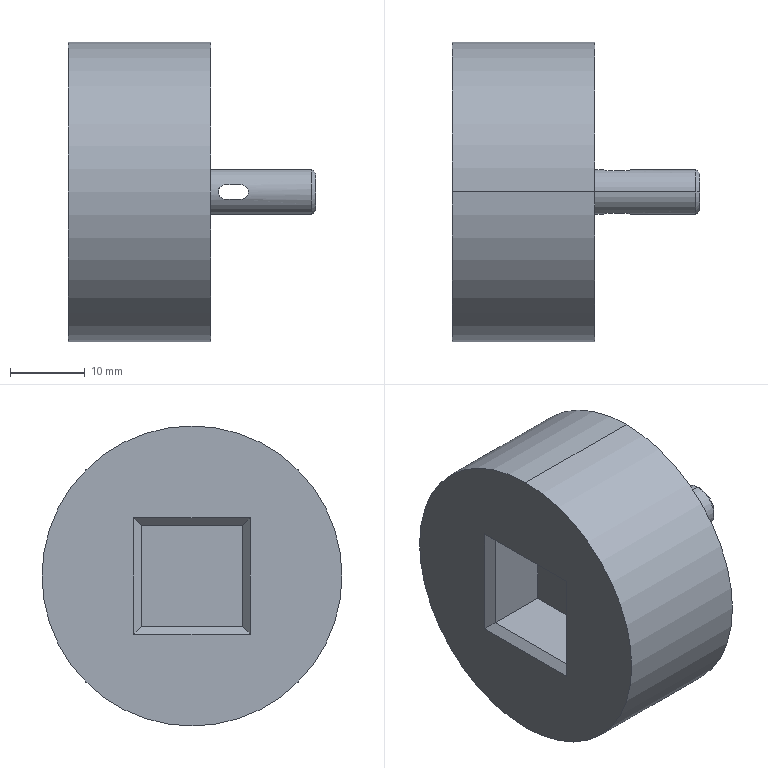Part | SolidWorks | features Chamfer 2, ICE 2, Revolution 1 | 1 solid | 22 faces | box 33 x 40 x 40 mm | volume 22559 mm3 | plane 14 | cylinder 6 | cone 2 | commonest cylinder face diameters 2 x2 6 x2 40 x2
STEP:
#1=CARTESIAN_POINT('',(14.,0.,-2.5));
#2=VERTEX_POINT('',#1);
#3=CARTESIAN_POINT('',(14.,0.,2.5));
#4=VERTEX_POINT('',#3);
#5=CARTESIAN_POINT('',(14.,0.,0.));
#6=DIRECTION('',(1.,0.,0.));
#7=DIRECTION('',(0.,0.,-1.));
#8=AXIS2_PLACEMENT_3D('',#5,#6,#7);
#9=CIRCLE('',#8,2.5);
#10=EDGE_CURVE('',#2,#4,#9,.T.);
#11=ORIENTED_EDGE('',*,*,#10,.F.);
#12=CARTESIAN_POINT('',(13.5,0.,-3.));
#13=VERTEX_POINT('',#12);
#14=CARTESIAN_POINT('',(13.5,0.,-3.));
#15=DIRECTION('',(-0.7071,0.,-0.7071));
#16=VECTOR('',#15,1000.);
#17=LINE('',#14,#16);
#18=EDGE_CURVE('',#2,#13,#17,.T.);
#19=ORIENTED_EDGE('',*,*,#18,.T.);
#20=CARTESIAN_POINT('',(13.5,0.,3.));
#21=VERTEX_POINT('',#20);
#22=CARTESIAN_POINT('',(13.5,0.,0.));
#23=DIRECTION('',(-1.,0.,0.));
#24=DIRECTION('',(0.,0.,-1.));
#25=AXIS2_PLACEMENT_3D('',#22,#23,#24);
#26=CIRCLE('',#25,3.);
#27=EDGE_CURVE('',#21,#13,#26,.T.);
#28=ORIENTED_EDGE('',*,*,#27,.F.);
#29=CARTESIAN_POINT('',(13.5,0.,3.));
#30=DIRECTION('',(-0.7071,0.,0.7071));
#31=VECTOR('',#30,1000.);
#32=LINE('',#29,#31);
#33=EDGE_CURVE('',#4,#21,#32,.T.);
#34=ORIENTED_EDGE('',*,*,#33,.F.);
#35=EDGE_LOOP('',(#11,#19,#28,#34));
#36=FACE_OUTER_BOUND('',#35,.T.);
#37=CARTESIAN_POINT('',(13.5,0.,0.));
#38=DIRECTION('',(-1.,0.,0.));
#39=DIRECTION('',(0.,0.,1.));
#40=AXIS2_PLACEMENT_3D('',#37,#38,#39);
#41=CONICAL_SURFACE('',#40,3.,0.7854);
#42=ADVANCED_FACE('',(#36),#41,.T.);
#43=CARTESIAN_POINT('',(2.,2.828,-1.));
#44=VERTEX_POINT('',#43);
#45=CARTESIAN_POINT('',(2.,2.828,1.));
#46=VERTEX_POINT('',#45);
#47=CARTESIAN_POINT('',(2.,2.828,-1.));
#48=CARTESIAN_POINT('',(1.867,2.828,-1.));
#49=CARTESIAN_POINT('',(1.736,2.838,-0.9735));
#50=CARTESIAN_POINT('',(1.495,2.871,-0.8728));
#51=CARTESIAN_POINT('',(1.384,2.893,-0.7987));
#52=CARTESIAN_POINT('',(1.201,2.938,-0.6157));
#53=CARTESIAN_POINT('',(1.127,2.96,-0.505));
#54=CARTESIAN_POINT('',(1.027,2.991,-0.2647));
#55=CARTESIAN_POINT('',(1.,3.,-0.1326));
#56=CARTESIAN_POINT('',(0.9999,3.,0.1304));
#57=CARTESIAN_POINT('',(1.026,2.991,0.2619));
#58=CARTESIAN_POINT('',(1.127,2.96,0.5053));
#59=CARTESIAN_POINT('',(1.201,2.938,0.6149));
#60=CARTESIAN_POINT('',(1.385,2.893,0.799));
#61=CARTESIAN_POINT('',(1.495,2.871,0.8728));
#62=CARTESIAN_POINT('',(1.735,2.838,0.9731));
#63=CARTESIAN_POINT('',(1.867,2.828,1.));
#64=CARTESIAN_POINT('',(2.,2.828,1.));
#65=B_SPLINE_CURVE_WITH_KNOTS('',3,(#47,#48,#49,#50,#51,#52,#53,#54,#55,#56,#57,#58,#59,#60,#61,#62,#63,#64),.UNSPECIFIED.,.F.,.F.,(4,2,2,2,2,2,2,2,4),(0.,0.0003935,0.000787,0.00118,0.001574,0.001967,0.002361,0.002754,0.003148),.UNSPECIFIED.);
#66=EDGE_CURVE('',#44,#46,#65,.T.);
#67=ORIENTED_EDGE('',*,*,#66,.F.);
#68=CARTESIAN_POINT('',(4.,2.828,-1.));
#69=VERTEX_POINT('',#68);
#70=CARTESIAN_POINT('',(-19.,2.828,-1.));
#71=DIRECTION('',(-1.,0.,0.));
#72=VECTOR('',#71,1000.);
#73=LINE('',#70,#72);
#74=EDGE_CURVE('',#69,#44,#73,.T.);
#75=ORIENTED_EDGE('',*,*,#74,.F.);
#76=CARTESIAN_POINT('',(4.,2.828,1.));
#77=VERTEX_POINT('',#76);
#78=CARTESIAN_POINT('',(4.,2.828,1.));
#79=CARTESIAN_POINT('',(4.133,2.828,1.));
#80=CARTESIAN_POINT('',(4.264,2.838,0.9735));
#81=CARTESIAN_POINT('',(4.505,2.871,0.8728));
#82=CARTESIAN_POINT('',(4.616,2.893,0.7987));
#83=CARTESIAN_POINT('',(4.799,2.938,0.6157));
#84=CARTESIAN_POINT('',(4.873,2.96,0.505));
#85=CARTESIAN_POINT('',(4.973,2.991,0.2647));
#86=CARTESIAN_POINT('',(5.,3.,0.1326));
#87=CARTESIAN_POINT('',(5.,3.,-0.1304));
#88=CARTESIAN_POINT('',(4.974,2.991,-0.2619));
#89=CARTESIAN_POINT('',(4.873,2.96,-0.5053));
#90=CARTESIAN_POINT('',(4.799,2.938,-0.6149));
#91=CARTESIAN_POINT('',(4.615,2.893,-0.799));
#92=CARTESIAN_POINT('',(4.505,2.871,-0.8728));
#93=CARTESIAN_POINT('',(4.265,2.838,-0.9731));
#94=CARTESIAN_POINT('',(4.133,2.828,-1.));
#95=CARTESIAN_POINT('',(4.,2.828,-1.));
#96=B_SPLINE_CURVE_WITH_KNOTS('',3,(#78,#79,#80,#81,#82,#83,#84,#85,#86,#87,#88,#89,#90,#91,#92,#93,#94,#95),.UNSPECIFIED.,.F.,.F.,(4,2,2,2,2,2,2,2,4),(0.,0.0003935,0.000787,0.00118,0.001574,0.001967,0.002361,0.002754,0.003148),.UNSPECIFIED.);
#97=EDGE_CURVE('',#77,#69,#96,.T.);
#98=ORIENTED_EDGE('',*,*,#97,.F.);
#99=CARTESIAN_POINT('',(-19.,2.828,1.));
#100=DIRECTION('',(1.,0.,0.));
#101=VECTOR('',#100,1000.);
#102=LINE('',#99,#101);
#103=EDGE_CURVE('',#46,#77,#102,.T.);
#104=ORIENTED_EDGE('',*,*,#103,.F.);
#105=EDGE_LOOP('',(#67,#75,#98,#104));
#106=FACE_BOUND('',#105,.T.);
#107=ORIENTED_EDGE('',*,*,#27,.T.);
#108=CARTESIAN_POINT('',(0.,0.,-3.));
#109=VERTEX_POINT('',#108);
#110=CARTESIAN_POINT('',(-19.,0.,-3.));
#111=DIRECTION('',(-1.,0.,0.));
#112=VECTOR('',#111,1000.);
#113=LINE('',#110,#112);
#114=EDGE_CURVE('',#13,#109,#113,.T.);
#115=ORIENTED_EDGE('',*,*,#114,.T.);
#116=CARTESIAN_POINT('',(0.,0.,3.));
#117=VERTEX_POINT('',#116);
#118=CARTESIAN_POINT('',(0.,0.,0.));
#119=DIRECTION('',(-1.,0.,0.));
#120=DIRECTION('',(0.,0.,1.));
#121=AXIS2_PLACEMENT_3D('',#118,#119,#120);
#122=CIRCLE('',#121,3.);
#123=EDGE_CURVE('',#117,#109,#122,.T.);
#124=ORIENTED_EDGE('',*,*,#123,.F.);
#125=CARTESIAN_POINT('',(-19.,0.,3.));
#126=DIRECTION('',(-1.,0.,0.));
#127=VECTOR('',#126,1000.);
#128=LINE('',#125,#127);
#129=EDGE_CURVE('',#21,#117,#128,.T.);
#130=ORIENTED_EDGE('',*,*,#129,.F.);
#131=EDGE_LOOP('',(#107,#115,#124,#130));
#132=FACE_OUTER_BOUND('',#131,.T.);
#133=CARTESIAN_POINT('',(-19.,0.,0.));
#134=DIRECTION('',(-1.,0.,0.));
#135=DIRECTION('',(0.,0.,1.));
#136=AXIS2_PLACEMENT_3D('',#133,#134,#135);
#137=CYLINDRICAL_SURFACE('',#136,3.);
#138=ADVANCED_FACE('',(#106,#132),#137,.T.);
#139=CARTESIAN_POINT('',(0.,0.,20.));
#140=VERTEX_POINT('',#139);
#141=CARTESIAN_POINT('',(0.,0.,-20.));
#142=VERTEX_POINT('',#141);
#143=CARTESIAN_POINT('',(0.,0.,0.));
#144=DIRECTION('',(-1.,0.,0.));
#145=DIRECTION('',(0.,0.,1.));
#146=AXIS2_PLACEMENT_3D('',#143,#144,#145);
#147=CIRCLE('',#146,20.);
#148=EDGE_CURVE('',#140,#142,#147,.T.);
#149=ORIENTED_EDGE('',*,*,#148,.T.);
#150=CARTESIAN_POINT('',(-19.,0.,-20.));
#151=VERTEX_POINT('',#150);
#152=CARTESIAN_POINT('',(-19.,0.,-20.));
#153=DIRECTION('',(-1.,0.,0.));
#154=VECTOR('',#153,1000.);
#155=LINE('',#152,#154);
#156=EDGE_CURVE('',#142,#151,#155,.T.);
#157=ORIENTED_EDGE('',*,*,#156,.T.);
#158=CARTESIAN_POINT('',(-19.,0.,20.));
#159=VERTEX_POINT('',#158);
#160=CARTESIAN_POINT('',(-19.,0.,0.));
#161=DIRECTION('',(-1.,0.,0.));
#162=DIRECTION('',(0.,0.,1.));
#163=AXIS2_PLACEMENT_3D('',#160,#161,#162);
#164=CIRCLE('',#163,20.);
#165=EDGE_CURVE('',#159,#151,#164,.T.);
#166=ORIENTED_EDGE('',*,*,#165,.F.);
#167=CARTESIAN_POINT('',(-19.,0.,20.));
#168=DIRECTION('',(-1.,0.,0.));
#169=VECTOR('',#168,1000.);
#170=LINE('',#167,#169);
#171=EDGE_CURVE('',#140,#159,#170,.T.);
#172=ORIENTED_EDGE('',*,*,#171,.F.);
#173=EDGE_LOOP('',(#149,#157,#166,#172));
#174=FACE_OUTER_BOUND('',#173,.T.);
#175=CARTESIAN_POINT('',(-19.,0.,0.));
#176=DIRECTION('',(-1.,0.,0.));
#177=DIRECTION('',(0.,0.,1.));
#178=AXIS2_PLACEMENT_3D('',#175,#176,#177);
#179=CYLINDRICAL_SURFACE('',#178,20.);
#180=ADVANCED_FACE('',(#174),#179,.T.);
#181=CARTESIAN_POINT('',(-19.,7.75,-7.75));
#182=VERTEX_POINT('',#181);
#183=CARTESIAN_POINT('',(-19.,7.75,7.75));
#184=VERTEX_POINT('',#183);
#185=CARTESIAN_POINT('',(-19.,7.75,0.));
#186=DIRECTION('',(0.,0.,1.));
#187=VECTOR('',#186,1000.);
#188=LINE('',#185,#187);
#189=EDGE_CURVE('',#182,#184,#188,.T.);
#190=ORIENTED_EDGE('',*,*,#189,.T.);
#191=CARTESIAN_POINT('',(-19.,-7.75,7.75));
#192=VERTEX_POINT('',#191);
#193=CARTESIAN_POINT('',(-19.,0.,7.75));
#194=DIRECTION('',(0.,-1.,0.));
#195=VECTOR('',#194,1000.);
#196=LINE('',#193,#195);
#197=EDGE_CURVE('',#184,#192,#196,.T.);
#198=ORIENTED_EDGE('',*,*,#197,.T.);
#199=CARTESIAN_POINT('',(-19.,-7.75,-7.75));
#200=VERTEX_POINT('',#199);
#201=CARTESIAN_POINT('',(-19.,-7.75,0.));
#202=DIRECTION('',(0.,0.,-1.));
#203=VECTOR('',#202,1000.);
#204=LINE('',#201,#203);
#205=EDGE_CURVE('',#192,#200,#204,.T.);
#206=ORIENTED_EDGE('',*,*,#205,.T.);
#207=CARTESIAN_POINT('',(-19.,0.,-7.75));
#208=DIRECTION('',(0.,1.,0.));
#209=VECTOR('',#208,1000.);
#210=LINE('',#207,#209);
#211=EDGE_CURVE('',#200,#182,#210,.T.);
#212=ORIENTED_EDGE('',*,*,#211,.T.);
#213=EDGE_LOOP('',(#190,#198,#206,#212));
#214=FACE_BOUND('',#213,.T.);
#215=ORIENTED_EDGE('',*,*,#165,.T.);
#216=CARTESIAN_POINT('',(-19.,0.,0.));
#217=DIRECTION('',(-1.,0.,0.));
#218=DIRECTION('',(0.,0.,1.));
#219=AXIS2_PLACEMENT_3D('',#216,#217,#218);
#220=CIRCLE('',#219,20.);
#221=EDGE_CURVE('',#151,#159,#220,.T.);
#222=ORIENTED_EDGE('',*,*,#221,.T.);
#223=EDGE_LOOP('',(#215,#222));
#224=FACE_OUTER_BOUND('',#223,.T.);
#225=CARTESIAN_POINT('',(-19.,0.,0.));
#226=DIRECTION('',(-1.,0.,0.));
#227=DIRECTION('',(0.,0.,1.));
#228=AXIS2_PLACEMENT_3D('',#225,#226,#227);
#229=PLANE('',#228);
#230=ADVANCED_FACE('',(#214,#224),#229,.T.);
#231=ORIENTED_EDGE('',*,*,#156,.F.);
#232=CARTESIAN_POINT('',(0.,0.,0.));
#233=DIRECTION('',(-1.,0.,0.));
#234=DIRECTION('',(0.,0.,1.));
#235=AXIS2_PLACEMENT_3D('',#232,#233,#234);
#236=CIRCLE('',#235,20.);
#237=EDGE_CURVE('',#142,#140,#236,.T.);
#238=ORIENTED_EDGE('',*,*,#237,.T.);
#239=ORIENTED_EDGE('',*,*,#171,.T.);
#240=ORIENTED_EDGE('',*,*,#221,.F.);
#241=EDGE_LOOP('',(#231,#238,#239,#240));
#242=FACE_OUTER_BOUND('',#241,.T.);
#243=CARTESIAN_POINT('',(-19.,0.,0.));
#244=DIRECTION('',(-1.,0.,0.));
#245=DIRECTION('',(0.,0.,1.));
#246=AXIS2_PLACEMENT_3D('',#243,#244,#245);
#247=CYLINDRICAL_SURFACE('',#246,20.);
#248=ADVANCED_FACE('',(#242),#247,.T.);
#249=ORIENTED_EDGE('',*,*,#123,.T.);
#250=CARTESIAN_POINT('',(0.,0.,0.));
#251=DIRECTION('',(-1.,0.,0.));
#252=DIRECTION('',(0.,0.,1.));
#253=AXIS2_PLACEMENT_3D('',#250,#251,#252);
#254=CIRCLE('',#253,3.);
#255=EDGE_CURVE('',#109,#117,#254,.T.);
#256=ORIENTED_EDGE('',*,*,#255,.T.);
#257=EDGE_LOOP('',(#249,#256));
#258=FACE_BOUND('',#257,.T.);
#259=ORIENTED_EDGE('',*,*,#148,.F.);
#260=ORIENTED_EDGE('',*,*,#237,.F.);
#261=EDGE_LOOP('',(#259,#260));
#262=FACE_OUTER_BOUND('',#261,.T.);
#263=CARTESIAN_POINT('',(0.,0.,3.));
#264=DIRECTION('',(1.,0.,0.));
#265=DIRECTION('',(0.,0.,-1.));
#266=AXIS2_PLACEMENT_3D('',#263,#264,#265);
#267=PLANE('',#266);
#268=ADVANCED_FACE('',(#258,#262),#267,.T.);
#269=ORIENTED_EDGE('',*,*,#114,.F.);
#270=CARTESIAN_POINT('',(13.5,0.,0.));
#271=DIRECTION('',(-1.,0.,0.));
#272=DIRECTION('',(0.,0.,-1.));
#273=AXIS2_PLACEMENT_3D('',#270,#271,#272);
#274=CIRCLE('',#273,3.);
#275=EDGE_CURVE('',#13,#21,#274,.T.);
#276=ORIENTED_EDGE('',*,*,#275,.T.);
#277=ORIENTED_EDGE('',*,*,#129,.T.);
#278=ORIENTED_EDGE('',*,*,#255,.F.);
#279=EDGE_LOOP('',(#269,#276,#277,#278));
#280=FACE_OUTER_BOUND('',#279,.T.);
#281=CARTESIAN_POINT('',(2.,-2.828,1.));
#282=VERTEX_POINT('',#281);
#283=CARTESIAN_POINT('',(2.,-2.828,-1.));
#284=VERTEX_POINT('',#283);
#285=CARTESIAN_POINT('',(2.,-2.828,1.));
#286=CARTESIAN_POINT('',(1.867,-2.828,1.));
#287=CARTESIAN_POINT('',(1.736,-2.838,0.9735));
#288=CARTESIAN_POINT('',(1.495,-2.871,0.8728));
#289=CARTESIAN_POINT('',(1.384,-2.893,0.7987));
#290=CARTESIAN_POINT('',(1.201,-2.938,0.6157));
#291=CARTESIAN_POINT('',(1.127,-2.96,0.505));
#292=CARTESIAN_POINT('',(1.027,-2.991,0.2647));
#293=CARTESIAN_POINT('',(1.,-3.,0.1326));
#294=CARTESIAN_POINT('',(0.9999,-3.,-0.1304));
#295=CARTESIAN_POINT('',(1.026,-2.991,-0.2619));
#296=CARTESIAN_POINT('',(1.127,-2.96,-0.5053));
#297=CARTESIAN_POINT('',(1.201,-2.938,-0.6149));
#298=CARTESIAN_POINT('',(1.385,-2.893,-0.799));
#299=CARTESIAN_POINT('',(1.495,-2.871,-0.8728));
#300=CARTESIAN_POINT('',(1.735,-2.838,-0.9731));
#301=CARTESIAN_POINT('',(1.867,-2.828,-1.));
#302=CARTESIAN_POINT('',(2.,-2.828,-1.));
#303=B_SPLINE_CURVE_WITH_KNOTS('',3,(#285,#286,#287,#288,#289,#290,#291,#292,#293,#294,#295,#296,#297,#298,#299,#300,#301,#302),.UNSPECIFIED.,.F.,.F.,(4,2,2,2,2,2,2,2,4),(0.,0.0003935,0.000787,0.00118,0.001574,0.001967,0.002361,0.002754,0.003148),.UNSPECIFIED.);
#304=EDGE_CURVE('',#282,#284,#303,.T.);
#305=ORIENTED_EDGE('',*,*,#304,.F.);
#306=CARTESIAN_POINT('',(4.,-2.828,1.));
#307=VERTEX_POINT('',#306);
#308=CARTESIAN_POINT('',(-19.,-2.828,1.));
#309=DIRECTION('',(-1.,0.,0.));
#310=VECTOR('',#309,1000.);
#311=LINE('',#308,#310);
#312=EDGE_CURVE('',#307,#282,#311,.T.);
#313=ORIENTED_EDGE('',*,*,#312,.F.);
#314=CARTESIAN_POINT('',(4.,-2.828,-1.));
#315=VERTEX_POINT('',#314);
#316=CARTESIAN_POINT('',(4.,-2.828,-1.));
#317=CARTESIAN_POINT('',(4.133,-2.828,-1.));
#318=CARTESIAN_POINT('',(4.264,-2.838,-0.9735));
#319=CARTESIAN_POINT('',(4.505,-2.871,-0.8728));
#320=CARTESIAN_POINT('',(4.616,-2.893,-0.7987));
#321=CARTESIAN_POINT('',(4.799,-2.938,-0.6157));
#322=CARTESIAN_POINT('',(4.873,-2.96,-0.505));
#323=CARTESIAN_POINT('',(4.973,-2.991,-0.2647));
#324=CARTESIAN_POINT('',(5.,-3.,-0.1326));
#325=CARTESIAN_POINT('',(5.,-3.,0.1304));
#326=CARTESIAN_POINT('',(4.974,-2.991,0.2619));
#327=CARTESIAN_POINT('',(4.873,-2.96,0.5053));
#328=CARTESIAN_POINT('',(4.799,-2.938,0.6149));
#329=CARTESIAN_POINT('',(4.615,-2.893,0.799));
#330=CARTESIAN_POINT('',(4.505,-2.871,0.8728));
#331=CARTESIAN_POINT('',(4.265,-2.838,0.9731));
#332=CARTESIAN_POINT('',(4.133,-2.828,1.));
#333=CARTESIAN_POINT('',(4.,-2.828,1.));
#334=B_SPLINE_CURVE_WITH_KNOTS('',3,(#316,#317,#318,#319,#320,#321,#322,#323,#324,#325,#326,#327,#328,#329,#330,#331,#332,#333),.UNSPECIFIED.,.F.,.F.,(4,2,2,2,2,2,2,2,4),(0.,0.0003935,0.000787,0.00118,0.001574,0.001967,0.002361,0.002754,0.003148),.UNSPECIFIED.);
#335=EDGE_CURVE('',#315,#307,#334,.T.);
#336=ORIENTED_EDGE('',*,*,#335,.F.);
#337=CARTESIAN_POINT('',(-19.,-2.828,-1.));
#338=DIRECTION('',(1.,0.,0.));
#339=VECTOR('',#338,1000.);
#340=LINE('',#337,#339);
#341=EDGE_CURVE('',#284,#315,#340,.T.);
#342=ORIENTED_EDGE('',*,*,#341,.F.);
#343=EDGE_LOOP('',(#305,#313,#336,#342));
#344=FACE_BOUND('',#343,.T.);
#345=CARTESIAN_POINT('',(-19.,0.,0.));
#346=DIRECTION('',(-1.,0.,0.));
#347=DIRECTION('',(0.,0.,1.));
#348=AXIS2_PLACEMENT_3D('',#345,#346,#347);
#349=CYLINDRICAL_SURFACE('',#348,3.);
#350=ADVANCED_FACE('',(#280,#344),#349,.T.);
#351=CARTESIAN_POINT('',(14.,0.,0.));
#352=DIRECTION('',(1.,0.,0.));
#353=DIRECTION('',(0.,0.,-1.));
#354=AXIS2_PLACEMENT_3D('',#351,#352,#353);
#355=CIRCLE('',#354,2.5);
#356=EDGE_CURVE('',#4,#2,#355,.T.);
#357=ORIENTED_EDGE('',*,*,#356,.T.);
#358=ORIENTED_EDGE('',*,*,#10,.T.);
#359=EDGE_LOOP('',(#357,#358));
#360=FACE_OUTER_BOUND('',#359,.T.);
#361=CARTESIAN_POINT('',(14.,0.,3.));
#362=DIRECTION('',(1.,0.,0.));
#363=DIRECTION('',(0.,0.,-1.));
#364=AXIS2_PLACEMENT_3D('',#361,#362,#363);
#365=PLANE('',#364);
#366=ADVANCED_FACE('',(#360),#365,.T.);
#367=CARTESIAN_POINT('',(-10.,-6.75,6.75));
#368=VERTEX_POINT('',#367);
#369=CARTESIAN_POINT('',(-18.,-6.75,6.75));
#370=VERTEX_POINT('',#369);
#371=CARTESIAN_POINT('',(-10.,-6.75,6.75));
#372=DIRECTION('',(-1.,0.,0.));
#373=VECTOR('',#372,1000.);
#374=LINE('',#371,#373);
#375=EDGE_CURVE('',#368,#370,#374,.T.);
#376=ORIENTED_EDGE('',*,*,#375,.T.);
#377=CARTESIAN_POINT('',(-18.,6.75,6.75));
#378=VERTEX_POINT('',#377);
#379=CARTESIAN_POINT('',(-18.,-6.75,6.75));
#380=DIRECTION('',(0.,1.,0.));
#381=VECTOR('',#380,1000.);
#382=LINE('',#379,#381);
#383=EDGE_CURVE('',#370,#378,#382,.T.);
#384=ORIENTED_EDGE('',*,*,#383,.T.);
#385=CARTESIAN_POINT('',(-10.,6.75,6.75));
#386=VERTEX_POINT('',#385);
#387=CARTESIAN_POINT('',(-10.,6.75,6.75));
#388=DIRECTION('',(-1.,0.,0.));
#389=VECTOR('',#388,1000.);
#390=LINE('',#387,#389);
#391=EDGE_CURVE('',#386,#378,#390,.T.);
#392=ORIENTED_EDGE('',*,*,#391,.F.);
#393=CARTESIAN_POINT('',(-10.,-6.75,6.75));
#394=DIRECTION('',(0.,-1.,0.));
#395=VECTOR('',#394,1000.);
#396=LINE('',#393,#395);
#397=EDGE_CURVE('',#386,#368,#396,.T.);
#398=ORIENTED_EDGE('',*,*,#397,.T.);
#399=EDGE_LOOP('',(#376,#384,#392,#398));
#400=FACE_OUTER_BOUND('',#399,.T.);
#401=CARTESIAN_POINT('',(-10.,-6.75,6.75));
#402=DIRECTION('',(0.,0.,-1.));
#403=DIRECTION('',(-1.,0.,0.));
#404=AXIS2_PLACEMENT_3D('',#401,#402,#403);
#405=PLANE('',#404);
#406=ADVANCED_FACE('',(#400),#405,.T.);
#407=CARTESIAN_POINT('',(-10.,-6.75,-6.75));
#408=VERTEX_POINT('',#407);
#409=CARTESIAN_POINT('',(-18.,-6.75,-6.75));
#410=VERTEX_POINT('',#409);
#411=CARTESIAN_POINT('',(-10.,-6.75,-6.75));
#412=DIRECTION('',(-1.,0.,0.));
#413=VECTOR('',#412,1000.);
#414=LINE('',#411,#413);
#415=EDGE_CURVE('',#408,#410,#414,.T.);
#416=ORIENTED_EDGE('',*,*,#415,.T.);
#417=CARTESIAN_POINT('',(-18.,-6.75,-6.75));
#418=DIRECTION('',(0.,0.,1.));
#419=VECTOR('',#418,1000.);
#420=LINE('',#417,#419);
#421=EDGE_CURVE('',#410,#370,#420,.T.);
#422=ORIENTED_EDGE('',*,*,#421,.T.);
#423=ORIENTED_EDGE('',*,*,#375,.F.);
#424=CARTESIAN_POINT('',(-10.,-6.75,-6.75));
#425=DIRECTION('',(0.,0.,-1.));
#426=VECTOR('',#425,1000.);
#427=LINE('',#424,#426);
#428=EDGE_CURVE('',#368,#408,#427,.T.);
#429=ORIENTED_EDGE('',*,*,#428,.T.);
#430=EDGE_LOOP('',(#416,#422,#423,#429));
#431=FACE_OUTER_BOUND('',#430,.T.);
#432=CARTESIAN_POINT('',(-10.,-6.75,-6.75));
#433=DIRECTION('',(0.,1.,0.));
#434=DIRECTION('',(0.,0.,1.));
#435=AXIS2_PLACEMENT_3D('',#432,#433,#434);
#436=PLANE('',#435);
#437=ADVANCED_FACE('',(#431),#436,.T.);
#438=CARTESIAN_POINT('',(-10.,6.75,-6.75));
#439=VERTEX_POINT('',#438);
#440=CARTESIAN_POINT('',(-18.,6.75,-6.75));
#441=VERTEX_POINT('',#440);
#442=CARTESIAN_POINT('',(-10.,6.75,-6.75));
#443=DIRECTION('',(-1.,0.,0.));
#444=VECTOR('',#443,1000.);
#445=LINE('',#442,#444);
#446=EDGE_CURVE('',#439,#441,#445,.T.);
#447=ORIENTED_EDGE('',*,*,#446,.T.);
#448=CARTESIAN_POINT('',(-18.,-6.75,-6.75));
#449=DIRECTION('',(0.,-1.,0.));
#450=VECTOR('',#449,1000.);
#451=LINE('',#448,#450);
#452=EDGE_CURVE('',#441,#410,#451,.T.);
#453=ORIENTED_EDGE('',*,*,#452,.T.);
#454=ORIENTED_EDGE('',*,*,#415,.F.);
#455=CARTESIAN_POINT('',(-10.,-6.75,-6.75));
#456=DIRECTION('',(0.,1.,0.));
#457=VECTOR('',#456,1000.);
#458=LINE('',#455,#457);
#459=EDGE_CURVE('',#408,#439,#458,.T.);
#460=ORIENTED_EDGE('',*,*,#459,.T.);
#461=EDGE_LOOP('',(#447,#453,#454,#460));
#462=FACE_OUTER_BOUND('',#461,.T.);
#463=CARTESIAN_POINT('',(-10.,-6.75,-6.75));
#464=DIRECTION('',(0.,0.,1.));
#465=DIRECTION('',(1.,0.,0.));
#466=AXIS2_PLACEMENT_3D('',#463,#464,#465);
#467=PLANE('',#466);
#468=ADVANCED_FACE('',(#462),#467,.T.);
#469=ORIENTED_EDGE('',*,*,#391,.T.);
#470=CARTESIAN_POINT('',(-18.,6.75,-6.75));
#471=DIRECTION('',(0.,0.,-1.));
#472=VECTOR('',#471,1000.);
#473=LINE('',#470,#472);
#474=EDGE_CURVE('',#378,#441,#473,.T.);
#475=ORIENTED_EDGE('',*,*,#474,.T.);
#476=ORIENTED_EDGE('',*,*,#446,.F.);
#477=CARTESIAN_POINT('',(-10.,6.75,-6.75));
#478=DIRECTION('',(0.,0.,1.));
#479=VECTOR('',#478,1000.);
#480=LINE('',#477,#479);
#481=EDGE_CURVE('',#439,#386,#480,.T.);
#482=ORIENTED_EDGE('',*,*,#481,.T.);
#483=EDGE_LOOP('',(#469,#475,#476,#482));
#484=FACE_OUTER_BOUND('',#483,.T.);
#485=CARTESIAN_POINT('',(-10.,6.75,-6.75));
#486=DIRECTION('',(0.,-1.,0.));
#487=DIRECTION('',(0.,0.,-1.));
#488=AXIS2_PLACEMENT_3D('',#485,#486,#487);
#489=PLANE('',#488);
#490=ADVANCED_FACE('',(#484),#489,.T.);
#491=ORIENTED_EDGE('',*,*,#397,.F.);
#492=ORIENTED_EDGE('',*,*,#481,.F.);
#493=ORIENTED_EDGE('',*,*,#459,.F.);
#494=ORIENTED_EDGE('',*,*,#428,.F.);
#495=EDGE_LOOP('',(#491,#492,#493,#494));
#496=FACE_OUTER_BOUND('',#495,.T.);
#497=CARTESIAN_POINT('',(-10.,6.75,6.75));
#498=DIRECTION('',(1.,0.,0.));
#499=DIRECTION('',(0.,0.,-1.));
#500=AXIS2_PLACEMENT_3D('',#497,#498,#499);
#501=PLANE('',#500);
#502=ADVANCED_FACE('',(#496),#501,.F.);
#503=CARTESIAN_POINT('',(-16.417,-5.167,-5.167));
#504=DIRECTION('',(-0.5774,-0.5774,-0.5774));
#505=VECTOR('',#504,1000.);
#506=LINE('',#503,#505);
#507=EDGE_CURVE('',#410,#200,#506,.T.);
#508=ORIENTED_EDGE('',*,*,#507,.F.);
#509=ORIENTED_EDGE('',*,*,#452,.F.);
#510=CARTESIAN_POINT('',(-16.417,5.167,-5.167));
#511=DIRECTION('',(0.5774,-0.5774,0.5774));
#512=VECTOR('',#511,1000.);
#513=LINE('',#510,#512);
#514=EDGE_CURVE('',#182,#441,#513,.T.);
#515=ORIENTED_EDGE('',*,*,#514,.F.);
#516=ORIENTED_EDGE('',*,*,#211,.F.);
#517=EDGE_LOOP('',(#508,#509,#515,#516));
#518=FACE_OUTER_BOUND('',#517,.T.);
#519=CARTESIAN_POINT('',(-19.,0.,-7.75));
#520=DIRECTION('',(0.7071,0.,-0.7071));
#521=DIRECTION('',(-0.7071,0.,-0.7071));
#522=AXIS2_PLACEMENT_3D('',#519,#520,#521);
#523=PLANE('',#522);
#524=ADVANCED_FACE('',(#518),#523,.F.);
#525=ORIENTED_EDGE('',*,*,#514,.T.);
#526=ORIENTED_EDGE('',*,*,#474,.F.);
#527=CARTESIAN_POINT('',(-16.417,5.167,5.167));
#528=DIRECTION('',(0.5774,-0.5774,-0.5774));
#529=VECTOR('',#528,1000.);
#530=LINE('',#527,#529);
#531=EDGE_CURVE('',#184,#378,#530,.T.);
#532=ORIENTED_EDGE('',*,*,#531,.F.);
#533=ORIENTED_EDGE('',*,*,#189,.F.);
#534=EDGE_LOOP('',(#525,#526,#532,#533));
#535=FACE_OUTER_BOUND('',#534,.T.);
#536=CARTESIAN_POINT('',(-19.,7.75,0.));
#537=DIRECTION('',(0.7071,0.7071,0.));
#538=DIRECTION('',(-0.7071,0.7071,0.));
#539=AXIS2_PLACEMENT_3D('',#536,#537,#538);
#540=PLANE('',#539);
#541=ADVANCED_FACE('',(#535),#540,.F.);
#542=ORIENTED_EDGE('',*,*,#507,.T.);
#543=ORIENTED_EDGE('',*,*,#205,.F.);
#544=CARTESIAN_POINT('',(-16.417,-5.167,5.167));
#545=DIRECTION('',(-0.5774,-0.5774,0.5774));
#546=VECTOR('',#545,1000.);
#547=LINE('',#544,#546);
#548=EDGE_CURVE('',#370,#192,#547,.T.);
#549=ORIENTED_EDGE('',*,*,#548,.F.);
#550=ORIENTED_EDGE('',*,*,#421,.F.);
#551=EDGE_LOOP('',(#542,#543,#549,#550));
#552=FACE_OUTER_BOUND('',#551,.T.);
#553=CARTESIAN_POINT('',(-19.,-7.75,0.));
#554=DIRECTION('',(0.7071,-0.7071,0.));
#555=DIRECTION('',(0.7071,0.7071,0.));
#556=AXIS2_PLACEMENT_3D('',#553,#554,#555);
#557=PLANE('',#556);
#558=ADVANCED_FACE('',(#552),#557,.F.);
#559=ORIENTED_EDGE('',*,*,#531,.T.);
#560=ORIENTED_EDGE('',*,*,#383,.F.);
#561=ORIENTED_EDGE('',*,*,#548,.T.);
#562=ORIENTED_EDGE('',*,*,#197,.F.);
#563=EDGE_LOOP('',(#559,#560,#561,#562));
#564=FACE_OUTER_BOUND('',#563,.T.);
#565=CARTESIAN_POINT('',(-19.,0.,7.75));
#566=DIRECTION('',(0.7071,0.,0.7071));
#567=DIRECTION('',(0.7071,0.,-0.7071));
#568=AXIS2_PLACEMENT_3D('',#565,#566,#567);
#569=PLANE('',#568);
#570=ADVANCED_FACE('',(#564),#569,.F.);
#571=ORIENTED_EDGE('',*,*,#304,.T.);
#572=CARTESIAN_POINT('',(2.,-20.,-1.));
#573=DIRECTION('',(0.,1.,0.));
#574=VECTOR('',#573,1000.);
#575=LINE('',#572,#574);
#576=EDGE_CURVE('',#284,#44,#575,.T.);
#577=ORIENTED_EDGE('',*,*,#576,.T.);
#578=ORIENTED_EDGE('',*,*,#66,.T.);
#579=CARTESIAN_POINT('',(2.,-20.,1.));
#580=DIRECTION('',(0.,1.,0.));
#581=VECTOR('',#580,1000.);
#582=LINE('',#579,#581);
#583=EDGE_CURVE('',#282,#46,#582,.T.);
#584=ORIENTED_EDGE('',*,*,#583,.F.);
#585=EDGE_LOOP('',(#571,#577,#578,#584));
#586=FACE_OUTER_BOUND('',#585,.T.);
#587=CARTESIAN_POINT('',(2.,-20.,0.));
#588=DIRECTION('',(0.,1.,0.));
#589=DIRECTION('',(0.,0.,1.));
#590=AXIS2_PLACEMENT_3D('',#587,#588,#589);
#591=CYLINDRICAL_SURFACE('',#590,1.);
#592=ADVANCED_FACE('',(#586),#591,.F.);
#593=ORIENTED_EDGE('',*,*,#341,.T.);
#594=CARTESIAN_POINT('',(4.,-20.,-1.));
#595=DIRECTION('',(0.,1.,0.));
#596=VECTOR('',#595,1000.);
#597=LINE('',#594,#596);
#598=EDGE_CURVE('',#315,#69,#597,.T.);
#599=ORIENTED_EDGE('',*,*,#598,.T.);
#600=ORIENTED_EDGE('',*,*,#74,.T.);
#601=ORIENTED_EDGE('',*,*,#576,.F.);
#602=EDGE_LOOP('',(#593,#599,#600,#601));
#603=FACE_OUTER_BOUND('',#602,.T.);
#604=CARTESIAN_POINT('',(2.,-20.,-1.));
#605=DIRECTION('',(0.,0.,-1.));
#606=DIRECTION('',(-1.,0.,0.));
#607=AXIS2_PLACEMENT_3D('',#604,#605,#606);
#608=PLANE('',#607);
#609=ADVANCED_FACE('',(#603),#608,.F.);
#610=ORIENTED_EDGE('',*,*,#335,.T.);
#611=CARTESIAN_POINT('',(4.,-20.,1.));
#612=DIRECTION('',(0.,1.,0.));
#613=VECTOR('',#612,1000.);
#614=LINE('',#611,#613);
#615=EDGE_CURVE('',#307,#77,#614,.T.);
#616=ORIENTED_EDGE('',*,*,#615,.T.);
#617=ORIENTED_EDGE('',*,*,#97,.T.);
#618=ORIENTED_EDGE('',*,*,#598,.F.);
#619=EDGE_LOOP('',(#610,#616,#617,#618));
#620=FACE_OUTER_BOUND('',#619,.T.);
#621=CARTESIAN_POINT('',(4.,-20.,0.));
#622=DIRECTION('',(0.,1.,0.));
#623=DIRECTION('',(0.,0.,1.));
#624=AXIS2_PLACEMENT_3D('',#621,#622,#623);
#625=CYLINDRICAL_SURFACE('',#624,1.);
#626=ADVANCED_FACE('',(#620),#625,.F.);
#627=ORIENTED_EDGE('',*,*,#103,.T.);
#628=ORIENTED_EDGE('',*,*,#615,.F.);
#629=ORIENTED_EDGE('',*,*,#312,.T.);
#630=ORIENTED_EDGE('',*,*,#583,.T.);
#631=EDGE_LOOP('',(#627,#628,#629,#630));
#632=FACE_OUTER_BOUND('',#631,.T.);
#633=CARTESIAN_POINT('',(2.,-20.,1.));
#634=DIRECTION('',(0.,0.,1.));
#635=DIRECTION('',(1.,0.,0.));
#636=AXIS2_PLACEMENT_3D('',#633,#634,#635);
#637=PLANE('',#636);
#638=ADVANCED_FACE('',(#632),#637,.F.);
#639=ORIENTED_EDGE('',*,*,#18,.F.);
#640=ORIENTED_EDGE('',*,*,#356,.F.);
#641=ORIENTED_EDGE('',*,*,#33,.T.);
#642=ORIENTED_EDGE('',*,*,#275,.F.);
#643=EDGE_LOOP('',(#639,#640,#641,#642));
#644=FACE_OUTER_BOUND('',#643,.T.);
#645=CARTESIAN_POINT('',(13.5,0.,0.));
#646=DIRECTION('',(-1.,0.,0.));
#647=DIRECTION('',(0.,0.,1.));
#648=AXIS2_PLACEMENT_3D('',#645,#646,#647);
#649=CONICAL_SURFACE('',#648,3.,0.7854);
#650=ADVANCED_FACE('',(#644),#649,.T.);
#651=CLOSED_SHELL('',(#42,#138,#180,#230,#248,#268,#350,#366,#406,#437,#468,#490,#502,#524,#541,#558,#570,#592,#609,#626,#638,#650));
#652=MANIFOLD_SOLID_BREP('',#651);
#653=CARTESIAN_POINT('',(0.,0.,0.));
#654=DIRECTION('',(0.,0.,1.));
#655=DIRECTION('',(1.,0.,0.));
#656=AXIS2_PLACEMENT_3D('',#653,#654,#655);
#657=(LENGTH_UNIT()NAMED_UNIT(*)SI_UNIT(.MILLI.,.METRE.));
#658=UNCERTAINTY_MEASURE_WITH_UNIT(LENGTH_MEASURE(0.00001),#657,'','');
#659=(NAMED_UNIT(*)PLANE_ANGLE_UNIT()SI_UNIT($,.RADIAN.));
#660=(NAMED_UNIT(*)SI_UNIT($,.STERADIAN.)SOLID_ANGLE_UNIT());
#661=(GEOMETRIC_REPRESENTATION_CONTEXT(3)GLOBAL_UNCERTAINTY_ASSIGNED_CONTEXT((#658))GLOBAL_UNIT_ASSIGNED_CONTEXT((#657,#659,#660))REPRESENTATION_CONTEXT('',''));
#662=ADVANCED_BREP_SHAPE_REPRESENTATION('',(#652,#656),#661);